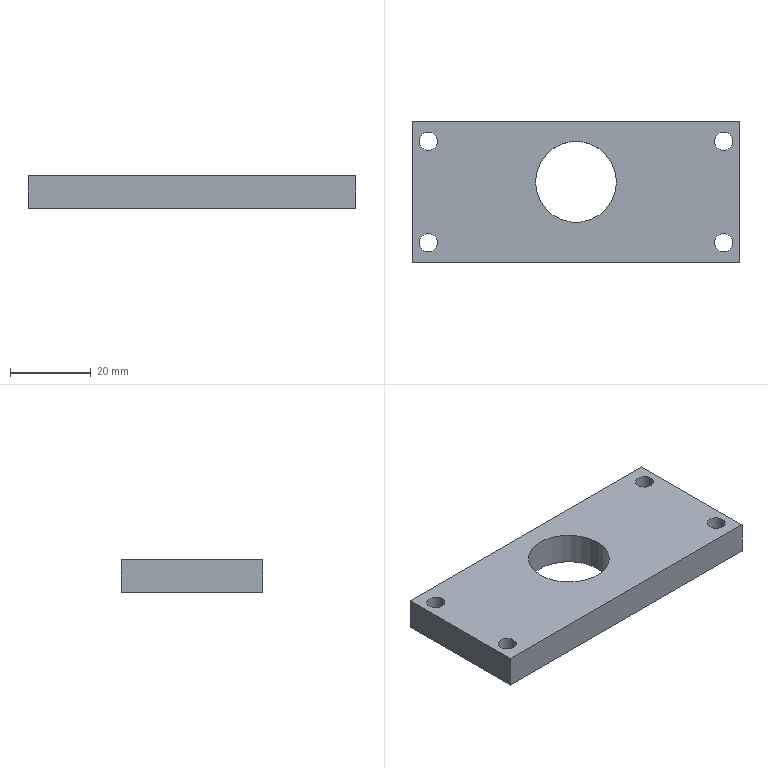Part | STEP file | slingshot push rod cylinder seat | 1 solid | 16 faces | box 81 x 35 x 8 mm | volume 19658 mm3 | cylinder 10 | plane 6 | commonest cylinder face diameters 4.5 x8 20 x2
STEP:
#1=CARTESIAN_POINT('',(0.,0.,0.));
#2=DIRECTION('',(0.,0.,1.));
#3=DIRECTION('',(1.,0.,0.));
#4=AXIS2_PLACEMENT_3D('',#1,#2,#3);
#5=CARTESIAN_POINT('',(-34.25,10.,0.));
#6=VERTEX_POINT('',#5);
#7=CARTESIAN_POINT('',(-34.25,10.,8.));
#8=VERTEX_POINT('',#7);
#9=CARTESIAN_POINT('',(-34.25,10.,-2.));
#10=DIRECTION('',(0.,0.,1.));
#11=VECTOR('',#10,1.);
#12=LINE('',#9,#11);
#13=CARTESIAN_POINT('',(-36.5,10.,-2.));
#14=DIRECTION('',(0.,0.,1.));
#15=DIRECTION('',(1.,0.,0.));
#16=AXIS2_PLACEMENT_3D('',#13,#14,#15);
#17=CYLINDRICAL_SURFACE('',#16,2.25);
#18=CARTESIAN_POINT('',(6.283,0.));
#19=DIRECTION('',(0.,1.));
#20=VECTOR('',#19,1.);
#21=LINE('',#18,#20);
#22=(GEOMETRIC_REPRESENTATION_CONTEXT(2)PARAMETRIC_REPRESENTATION_CONTEXT()REPRESENTATION_CONTEXT('',''));
#23=DEFINITIONAL_REPRESENTATION('',(#21),#22);
#24=PCURVE('',#17,#23);
#25=CARTESIAN_POINT('',(-36.5,10.,-2.));
#26=DIRECTION('',(0.,0.,1.));
#27=DIRECTION('',(1.,0.,0.));
#28=AXIS2_PLACEMENT_3D('',#25,#26,#27);
#29=CYLINDRICAL_SURFACE('',#28,2.25);
#30=CARTESIAN_POINT('',(0.,0.));
#31=DIRECTION('',(0.,1.));
#32=VECTOR('',#31,1.);
#33=LINE('',#30,#32);
#34=(GEOMETRIC_REPRESENTATION_CONTEXT(2)PARAMETRIC_REPRESENTATION_CONTEXT()REPRESENTATION_CONTEXT('',''));
#35=DEFINITIONAL_REPRESENTATION('',(#33),#34);
#36=PCURVE('',#29,#35);
#37=SURFACE_CURVE('',#12,(#24,#36),.PCURVE_S1.);
#38=EDGE_CURVE('',#6,#8,#37,.T.);
#39=ORIENTED_EDGE('',*,*,#38,.T.);
#40=CARTESIAN_POINT('',(-38.75,10.,8.));
#41=VERTEX_POINT('',#40);
#42=CARTESIAN_POINT('',(-36.5,10.,8.));
#43=DIRECTION('',(0.,0.,1.));
#44=DIRECTION('',(1.,0.,0.));
#45=AXIS2_PLACEMENT_3D('',#42,#43,#44);
#46=CIRCLE('',#45,2.25);
#47=CARTESIAN_POINT('',(0.,10.));
#48=DIRECTION('',(1.,0.));
#49=VECTOR('',#48,1.);
#50=LINE('',#47,#49);
#51=(GEOMETRIC_REPRESENTATION_CONTEXT(2)PARAMETRIC_REPRESENTATION_CONTEXT()REPRESENTATION_CONTEXT('',''));
#52=DEFINITIONAL_REPRESENTATION('',(#50),#51);
#53=PCURVE('',#17,#52);
#54=CARTESIAN_POINT('',(-40.5,-20.,8.));
#55=DIRECTION('',(0.,0.,1.));
#56=DIRECTION('',(1.,0.,0.));
#57=AXIS2_PLACEMENT_3D('',#54,#55,#56);
#58=PLANE('',#57);
#59=CARTESIAN_POINT('',(4.,30.));
#60=DIRECTION('',(1.,0.));
#61=AXIS2_PLACEMENT_2D('',#59,#60);
#62=CIRCLE('',#61,2.25);
#63=(GEOMETRIC_REPRESENTATION_CONTEXT(2)PARAMETRIC_REPRESENTATION_CONTEXT()REPRESENTATION_CONTEXT('',''));
#64=DEFINITIONAL_REPRESENTATION('',(#62),#63);
#65=PCURVE('',#58,#64);
#66=SURFACE_CURVE('',#46,(#53,#65),.PCURVE_S1.);
#67=EDGE_CURVE('',#41,#8,#66,.T.);
#68=ORIENTED_EDGE('',*,*,#67,.F.);
#69=CARTESIAN_POINT('',(-38.75,10.,0.));
#70=VERTEX_POINT('',#69);
#71=CARTESIAN_POINT('',(-38.75,10.,-2.));
#72=DIRECTION('',(0.,0.,1.));
#73=VECTOR('',#72,1.);
#74=LINE('',#71,#73);
#75=CARTESIAN_POINT('',(3.142,0.));
#76=DIRECTION('',(0.,1.));
#77=VECTOR('',#76,1.);
#78=LINE('',#75,#77);
#79=(GEOMETRIC_REPRESENTATION_CONTEXT(2)PARAMETRIC_REPRESENTATION_CONTEXT()REPRESENTATION_CONTEXT('',''));
#80=DEFINITIONAL_REPRESENTATION('',(#78),#79);
#81=PCURVE('',#17,#80);
#82=CARTESIAN_POINT('',(3.142,0.));
#83=DIRECTION('',(0.,1.));
#84=VECTOR('',#83,1.);
#85=LINE('',#82,#84);
#86=(GEOMETRIC_REPRESENTATION_CONTEXT(2)PARAMETRIC_REPRESENTATION_CONTEXT()REPRESENTATION_CONTEXT('',''));
#87=DEFINITIONAL_REPRESENTATION('',(#85),#86);
#88=PCURVE('',#29,#87);
#89=SURFACE_CURVE('',#74,(#81,#88),.PCURVE_S1.);
#90=EDGE_CURVE('',#70,#41,#89,.T.);
#91=ORIENTED_EDGE('',*,*,#90,.F.);
#92=CARTESIAN_POINT('',(-36.5,10.,0.));
#93=DIRECTION('',(0.,0.,1.));
#94=DIRECTION('',(1.,0.,0.));
#95=AXIS2_PLACEMENT_3D('',#92,#93,#94);
#96=CIRCLE('',#95,2.25);
#97=CARTESIAN_POINT('',(0.,2.));
#98=DIRECTION('',(1.,0.));
#99=VECTOR('',#98,1.);
#100=LINE('',#97,#99);
#101=(GEOMETRIC_REPRESENTATION_CONTEXT(2)PARAMETRIC_REPRESENTATION_CONTEXT()REPRESENTATION_CONTEXT('',''));
#102=DEFINITIONAL_REPRESENTATION('',(#100),#101);
#103=PCURVE('',#17,#102);
#104=CARTESIAN_POINT('',(-40.5,-20.,0.));
#105=DIRECTION('',(0.,0.,1.));
#106=DIRECTION('',(1.,0.,0.));
#107=AXIS2_PLACEMENT_3D('',#104,#105,#106);
#108=PLANE('',#107);
#109=CARTESIAN_POINT('',(4.,30.));
#110=DIRECTION('',(1.,0.));
#111=AXIS2_PLACEMENT_2D('',#109,#110);
#112=CIRCLE('',#111,2.25);
#113=(GEOMETRIC_REPRESENTATION_CONTEXT(2)PARAMETRIC_REPRESENTATION_CONTEXT()REPRESENTATION_CONTEXT('',''));
#114=DEFINITIONAL_REPRESENTATION('',(#112),#113);
#115=PCURVE('',#108,#114);
#116=SURFACE_CURVE('',#96,(#103,#115),.PCURVE_S1.);
#117=EDGE_CURVE('',#70,#6,#116,.T.);
#118=ORIENTED_EDGE('',*,*,#117,.T.);
#119=EDGE_LOOP('',(#39,#68,#91,#118));
#120=FACE_BOUND('',#119,.F.);
#121=ADVANCED_FACE('',(#120),#17,.F.);
#122=CARTESIAN_POINT('',(-34.25,-15.,0.));
#123=VERTEX_POINT('',#122);
#124=CARTESIAN_POINT('',(-34.25,-15.,8.));
#125=VERTEX_POINT('',#124);
#126=CARTESIAN_POINT('',(-34.25,-15.,-2.));
#127=DIRECTION('',(0.,0.,1.));
#128=VECTOR('',#127,1.);
#129=LINE('',#126,#128);
#130=CARTESIAN_POINT('',(-36.5,-15.,-2.));
#131=DIRECTION('',(0.,0.,1.));
#132=DIRECTION('',(1.,0.,0.));
#133=AXIS2_PLACEMENT_3D('',#130,#131,#132);
#134=CYLINDRICAL_SURFACE('',#133,2.25);
#135=CARTESIAN_POINT('',(6.283,0.));
#136=DIRECTION('',(0.,1.));
#137=VECTOR('',#136,1.);
#138=LINE('',#135,#137);
#139=(GEOMETRIC_REPRESENTATION_CONTEXT(2)PARAMETRIC_REPRESENTATION_CONTEXT()REPRESENTATION_CONTEXT('',''));
#140=DEFINITIONAL_REPRESENTATION('',(#138),#139);
#141=PCURVE('',#134,#140);
#142=CARTESIAN_POINT('',(-36.5,-15.,-2.));
#143=DIRECTION('',(0.,0.,1.));
#144=DIRECTION('',(1.,0.,0.));
#145=AXIS2_PLACEMENT_3D('',#142,#143,#144);
#146=CYLINDRICAL_SURFACE('',#145,2.25);
#147=CARTESIAN_POINT('',(0.,0.));
#148=DIRECTION('',(0.,1.));
#149=VECTOR('',#148,1.);
#150=LINE('',#147,#149);
#151=(GEOMETRIC_REPRESENTATION_CONTEXT(2)PARAMETRIC_REPRESENTATION_CONTEXT()REPRESENTATION_CONTEXT('',''));
#152=DEFINITIONAL_REPRESENTATION('',(#150),#151);
#153=PCURVE('',#146,#152);
#154=SURFACE_CURVE('',#129,(#141,#153),.PCURVE_S1.);
#155=EDGE_CURVE('',#123,#125,#154,.T.);
#156=ORIENTED_EDGE('',*,*,#155,.T.);
#157=CARTESIAN_POINT('',(-38.75,-15.,8.));
#158=VERTEX_POINT('',#157);
#159=CARTESIAN_POINT('',(-36.5,-15.,8.));
#160=DIRECTION('',(0.,0.,1.));
#161=DIRECTION('',(1.,0.,0.));
#162=AXIS2_PLACEMENT_3D('',#159,#160,#161);
#163=CIRCLE('',#162,2.25);
#164=CARTESIAN_POINT('',(0.,10.));
#165=DIRECTION('',(1.,0.));
#166=VECTOR('',#165,1.);
#167=LINE('',#164,#166);
#168=(GEOMETRIC_REPRESENTATION_CONTEXT(2)PARAMETRIC_REPRESENTATION_CONTEXT()REPRESENTATION_CONTEXT('',''));
#169=DEFINITIONAL_REPRESENTATION('',(#167),#168);
#170=PCURVE('',#134,#169);
#171=CARTESIAN_POINT('',(4.,5.));
#172=DIRECTION('',(1.,0.));
#173=AXIS2_PLACEMENT_2D('',#171,#172);
#174=CIRCLE('',#173,2.25);
#175=(GEOMETRIC_REPRESENTATION_CONTEXT(2)PARAMETRIC_REPRESENTATION_CONTEXT()REPRESENTATION_CONTEXT('',''));
#176=DEFINITIONAL_REPRESENTATION('',(#174),#175);
#177=PCURVE('',#58,#176);
#178=SURFACE_CURVE('',#163,(#170,#177),.PCURVE_S1.);
#179=EDGE_CURVE('',#158,#125,#178,.T.);
#180=ORIENTED_EDGE('',*,*,#179,.F.);
#181=CARTESIAN_POINT('',(-38.75,-15.,0.));
#182=VERTEX_POINT('',#181);
#183=CARTESIAN_POINT('',(-38.75,-15.,-2.));
#184=DIRECTION('',(0.,0.,1.));
#185=VECTOR('',#184,1.);
#186=LINE('',#183,#185);
#187=CARTESIAN_POINT('',(3.142,0.));
#188=DIRECTION('',(0.,1.));
#189=VECTOR('',#188,1.);
#190=LINE('',#187,#189);
#191=(GEOMETRIC_REPRESENTATION_CONTEXT(2)PARAMETRIC_REPRESENTATION_CONTEXT()REPRESENTATION_CONTEXT('',''));
#192=DEFINITIONAL_REPRESENTATION('',(#190),#191);
#193=PCURVE('',#134,#192);
#194=CARTESIAN_POINT('',(3.142,0.));
#195=DIRECTION('',(0.,1.));
#196=VECTOR('',#195,1.);
#197=LINE('',#194,#196);
#198=(GEOMETRIC_REPRESENTATION_CONTEXT(2)PARAMETRIC_REPRESENTATION_CONTEXT()REPRESENTATION_CONTEXT('',''));
#199=DEFINITIONAL_REPRESENTATION('',(#197),#198);
#200=PCURVE('',#146,#199);
#201=SURFACE_CURVE('',#186,(#193,#200),.PCURVE_S1.);
#202=EDGE_CURVE('',#182,#158,#201,.T.);
#203=ORIENTED_EDGE('',*,*,#202,.F.);
#204=CARTESIAN_POINT('',(-36.5,-15.,0.));
#205=DIRECTION('',(0.,0.,1.));
#206=DIRECTION('',(1.,0.,0.));
#207=AXIS2_PLACEMENT_3D('',#204,#205,#206);
#208=CIRCLE('',#207,2.25);
#209=CARTESIAN_POINT('',(0.,2.));
#210=DIRECTION('',(1.,0.));
#211=VECTOR('',#210,1.);
#212=LINE('',#209,#211);
#213=(GEOMETRIC_REPRESENTATION_CONTEXT(2)PARAMETRIC_REPRESENTATION_CONTEXT()REPRESENTATION_CONTEXT('',''));
#214=DEFINITIONAL_REPRESENTATION('',(#212),#213);
#215=PCURVE('',#134,#214);
#216=CARTESIAN_POINT('',(4.,5.));
#217=DIRECTION('',(1.,0.));
#218=AXIS2_PLACEMENT_2D('',#216,#217);
#219=CIRCLE('',#218,2.25);
#220=(GEOMETRIC_REPRESENTATION_CONTEXT(2)PARAMETRIC_REPRESENTATION_CONTEXT()REPRESENTATION_CONTEXT('',''));
#221=DEFINITIONAL_REPRESENTATION('',(#219),#220);
#222=PCURVE('',#108,#221);
#223=SURFACE_CURVE('',#208,(#215,#222),.PCURVE_S1.);
#224=EDGE_CURVE('',#182,#123,#223,.T.);
#225=ORIENTED_EDGE('',*,*,#224,.T.);
#226=EDGE_LOOP('',(#156,#180,#203,#225));
#227=FACE_BOUND('',#226,.F.);
#228=ADVANCED_FACE('',(#227),#134,.F.);
#229=CARTESIAN_POINT('',(38.75,-15.,0.));
#230=VERTEX_POINT('',#229);
#231=CARTESIAN_POINT('',(38.75,-15.,8.));
#232=VERTEX_POINT('',#231);
#233=CARTESIAN_POINT('',(38.75,-15.,-2.));
#234=DIRECTION('',(0.,0.,1.));
#235=VECTOR('',#234,1.);
#236=LINE('',#233,#235);
#237=CARTESIAN_POINT('',(36.5,-15.,-2.));
#238=DIRECTION('',(0.,0.,1.));
#239=DIRECTION('',(1.,0.,0.));
#240=AXIS2_PLACEMENT_3D('',#237,#238,#239);
#241=CYLINDRICAL_SURFACE('',#240,2.25);
#242=CARTESIAN_POINT('',(6.283,0.));
#243=DIRECTION('',(0.,1.));
#244=VECTOR('',#243,1.);
#245=LINE('',#242,#244);
#246=(GEOMETRIC_REPRESENTATION_CONTEXT(2)PARAMETRIC_REPRESENTATION_CONTEXT()REPRESENTATION_CONTEXT('',''));
#247=DEFINITIONAL_REPRESENTATION('',(#245),#246);
#248=PCURVE('',#241,#247);
#249=CARTESIAN_POINT('',(36.5,-15.,-2.));
#250=DIRECTION('',(0.,0.,1.));
#251=DIRECTION('',(1.,0.,0.));
#252=AXIS2_PLACEMENT_3D('',#249,#250,#251);
#253=CYLINDRICAL_SURFACE('',#252,2.25);
#254=CARTESIAN_POINT('',(0.,0.));
#255=DIRECTION('',(0.,1.));
#256=VECTOR('',#255,1.);
#257=LINE('',#254,#256);
#258=(GEOMETRIC_REPRESENTATION_CONTEXT(2)PARAMETRIC_REPRESENTATION_CONTEXT()REPRESENTATION_CONTEXT('',''));
#259=DEFINITIONAL_REPRESENTATION('',(#257),#258);
#260=PCURVE('',#253,#259);
#261=SURFACE_CURVE('',#236,(#248,#260),.PCURVE_S1.);
#262=EDGE_CURVE('',#230,#232,#261,.T.);
#263=ORIENTED_EDGE('',*,*,#262,.T.);
#264=CARTESIAN_POINT('',(34.25,-15.,8.));
#265=VERTEX_POINT('',#264);
#266=CARTESIAN_POINT('',(36.5,-15.,8.));
#267=DIRECTION('',(0.,0.,1.));
#268=DIRECTION('',(1.,0.,0.));
#269=AXIS2_PLACEMENT_3D('',#266,#267,#268);
#270=CIRCLE('',#269,2.25);
#271=CARTESIAN_POINT('',(0.,10.));
#272=DIRECTION('',(1.,0.));
#273=VECTOR('',#272,1.);
#274=LINE('',#271,#273);
#275=(GEOMETRIC_REPRESENTATION_CONTEXT(2)PARAMETRIC_REPRESENTATION_CONTEXT()REPRESENTATION_CONTEXT('',''));
#276=DEFINITIONAL_REPRESENTATION('',(#274),#275);
#277=PCURVE('',#241,#276);
#278=CARTESIAN_POINT('',(77.,5.));
#279=DIRECTION('',(1.,0.));
#280=AXIS2_PLACEMENT_2D('',#278,#279);
#281=CIRCLE('',#280,2.25);
#282=(GEOMETRIC_REPRESENTATION_CONTEXT(2)PARAMETRIC_REPRESENTATION_CONTEXT()REPRESENTATION_CONTEXT('',''));
#283=DEFINITIONAL_REPRESENTATION('',(#281),#282);
#284=PCURVE('',#58,#283);
#285=SURFACE_CURVE('',#270,(#277,#284),.PCURVE_S1.);
#286=EDGE_CURVE('',#265,#232,#285,.T.);
#287=ORIENTED_EDGE('',*,*,#286,.F.);
#288=CARTESIAN_POINT('',(34.25,-15.,0.));
#289=VERTEX_POINT('',#288);
#290=CARTESIAN_POINT('',(34.25,-15.,-2.));
#291=DIRECTION('',(0.,0.,1.));
#292=VECTOR('',#291,1.);
#293=LINE('',#290,#292);
#294=CARTESIAN_POINT('',(3.142,0.));
#295=DIRECTION('',(0.,1.));
#296=VECTOR('',#295,1.);
#297=LINE('',#294,#296);
#298=(GEOMETRIC_REPRESENTATION_CONTEXT(2)PARAMETRIC_REPRESENTATION_CONTEXT()REPRESENTATION_CONTEXT('',''));
#299=DEFINITIONAL_REPRESENTATION('',(#297),#298);
#300=PCURVE('',#241,#299);
#301=CARTESIAN_POINT('',(3.142,0.));
#302=DIRECTION('',(0.,1.));
#303=VECTOR('',#302,1.);
#304=LINE('',#301,#303);
#305=(GEOMETRIC_REPRESENTATION_CONTEXT(2)PARAMETRIC_REPRESENTATION_CONTEXT()REPRESENTATION_CONTEXT('',''));
#306=DEFINITIONAL_REPRESENTATION('',(#304),#305);
#307=PCURVE('',#253,#306);
#308=SURFACE_CURVE('',#293,(#300,#307),.PCURVE_S1.);
#309=EDGE_CURVE('',#289,#265,#308,.T.);
#310=ORIENTED_EDGE('',*,*,#309,.F.);
#311=CARTESIAN_POINT('',(36.5,-15.,0.));
#312=DIRECTION('',(0.,0.,1.));
#313=DIRECTION('',(1.,0.,0.));
#314=AXIS2_PLACEMENT_3D('',#311,#312,#313);
#315=CIRCLE('',#314,2.25);
#316=CARTESIAN_POINT('',(0.,2.));
#317=DIRECTION('',(1.,0.));
#318=VECTOR('',#317,1.);
#319=LINE('',#316,#318);
#320=(GEOMETRIC_REPRESENTATION_CONTEXT(2)PARAMETRIC_REPRESENTATION_CONTEXT()REPRESENTATION_CONTEXT('',''));
#321=DEFINITIONAL_REPRESENTATION('',(#319),#320);
#322=PCURVE('',#241,#321);
#323=CARTESIAN_POINT('',(77.,5.));
#324=DIRECTION('',(1.,0.));
#325=AXIS2_PLACEMENT_2D('',#323,#324);
#326=CIRCLE('',#325,2.25);
#327=(GEOMETRIC_REPRESENTATION_CONTEXT(2)PARAMETRIC_REPRESENTATION_CONTEXT()REPRESENTATION_CONTEXT('',''));
#328=DEFINITIONAL_REPRESENTATION('',(#326),#327);
#329=PCURVE('',#108,#328);
#330=SURFACE_CURVE('',#315,(#322,#329),.PCURVE_S1.);
#331=EDGE_CURVE('',#289,#230,#330,.T.);
#332=ORIENTED_EDGE('',*,*,#331,.T.);
#333=EDGE_LOOP('',(#263,#287,#310,#332));
#334=FACE_BOUND('',#333,.F.);
#335=ADVANCED_FACE('',(#334),#241,.F.);
#336=CARTESIAN_POINT('',(38.75,10.,0.));
#337=VERTEX_POINT('',#336);
#338=CARTESIAN_POINT('',(38.75,10.,8.));
#339=VERTEX_POINT('',#338);
#340=CARTESIAN_POINT('',(38.75,10.,-2.));
#341=DIRECTION('',(0.,0.,1.));
#342=VECTOR('',#341,1.);
#343=LINE('',#340,#342);
#344=CARTESIAN_POINT('',(36.5,10.,-2.));
#345=DIRECTION('',(0.,0.,1.));
#346=DIRECTION('',(1.,0.,0.));
#347=AXIS2_PLACEMENT_3D('',#344,#345,#346);
#348=CYLINDRICAL_SURFACE('',#347,2.25);
#349=CARTESIAN_POINT('',(6.283,0.));
#350=DIRECTION('',(0.,1.));
#351=VECTOR('',#350,1.);
#352=LINE('',#349,#351);
#353=(GEOMETRIC_REPRESENTATION_CONTEXT(2)PARAMETRIC_REPRESENTATION_CONTEXT()REPRESENTATION_CONTEXT('',''));
#354=DEFINITIONAL_REPRESENTATION('',(#352),#353);
#355=PCURVE('',#348,#354);
#356=CARTESIAN_POINT('',(36.5,10.,-2.));
#357=DIRECTION('',(0.,0.,1.));
#358=DIRECTION('',(1.,0.,0.));
#359=AXIS2_PLACEMENT_3D('',#356,#357,#358);
#360=CYLINDRICAL_SURFACE('',#359,2.25);
#361=CARTESIAN_POINT('',(0.,0.));
#362=DIRECTION('',(0.,1.));
#363=VECTOR('',#362,1.);
#364=LINE('',#361,#363);
#365=(GEOMETRIC_REPRESENTATION_CONTEXT(2)PARAMETRIC_REPRESENTATION_CONTEXT()REPRESENTATION_CONTEXT('',''));
#366=DEFINITIONAL_REPRESENTATION('',(#364),#365);
#367=PCURVE('',#360,#366);
#368=SURFACE_CURVE('',#343,(#355,#367),.PCURVE_S1.);
#369=EDGE_CURVE('',#337,#339,#368,.T.);
#370=ORIENTED_EDGE('',*,*,#369,.T.);
#371=CARTESIAN_POINT('',(34.25,10.,8.));
#372=VERTEX_POINT('',#371);
#373=CARTESIAN_POINT('',(36.5,10.,8.));
#374=DIRECTION('',(0.,0.,1.));
#375=DIRECTION('',(1.,0.,0.));
#376=AXIS2_PLACEMENT_3D('',#373,#374,#375);
#377=CIRCLE('',#376,2.25);
#378=CARTESIAN_POINT('',(0.,10.));
#379=DIRECTION('',(1.,0.));
#380=VECTOR('',#379,1.);
#381=LINE('',#378,#380);
#382=(GEOMETRIC_REPRESENTATION_CONTEXT(2)PARAMETRIC_REPRESENTATION_CONTEXT()REPRESENTATION_CONTEXT('',''));
#383=DEFINITIONAL_REPRESENTATION('',(#381),#382);
#384=PCURVE('',#348,#383);
#385=CARTESIAN_POINT('',(77.,30.));
#386=DIRECTION('',(1.,0.));
#387=AXIS2_PLACEMENT_2D('',#385,#386);
#388=CIRCLE('',#387,2.25);
#389=(GEOMETRIC_REPRESENTATION_CONTEXT(2)PARAMETRIC_REPRESENTATION_CONTEXT()REPRESENTATION_CONTEXT('',''));
#390=DEFINITIONAL_REPRESENTATION('',(#388),#389);
#391=PCURVE('',#58,#390);
#392=SURFACE_CURVE('',#377,(#384,#391),.PCURVE_S1.);
#393=EDGE_CURVE('',#372,#339,#392,.T.);
#394=ORIENTED_EDGE('',*,*,#393,.F.);
#395=CARTESIAN_POINT('',(34.25,10.,0.));
#396=VERTEX_POINT('',#395);
#397=CARTESIAN_POINT('',(34.25,10.,-2.));
#398=DIRECTION('',(0.,0.,1.));
#399=VECTOR('',#398,1.);
#400=LINE('',#397,#399);
#401=CARTESIAN_POINT('',(3.142,0.));
#402=DIRECTION('',(0.,1.));
#403=VECTOR('',#402,1.);
#404=LINE('',#401,#403);
#405=(GEOMETRIC_REPRESENTATION_CONTEXT(2)PARAMETRIC_REPRESENTATION_CONTEXT()REPRESENTATION_CONTEXT('',''));
#406=DEFINITIONAL_REPRESENTATION('',(#404),#405);
#407=PCURVE('',#348,#406);
#408=CARTESIAN_POINT('',(3.142,0.));
#409=DIRECTION('',(0.,1.));
#410=VECTOR('',#409,1.);
#411=LINE('',#408,#410);
#412=(GEOMETRIC_REPRESENTATION_CONTEXT(2)PARAMETRIC_REPRESENTATION_CONTEXT()REPRESENTATION_CONTEXT('',''));
#413=DEFINITIONAL_REPRESENTATION('',(#411),#412);
#414=PCURVE('',#360,#413);
#415=SURFACE_CURVE('',#400,(#407,#414),.PCURVE_S1.);
#416=EDGE_CURVE('',#396,#372,#415,.T.);
#417=ORIENTED_EDGE('',*,*,#416,.F.);
#418=CARTESIAN_POINT('',(36.5,10.,0.));
#419=DIRECTION('',(0.,0.,1.));
#420=DIRECTION('',(1.,0.,0.));
#421=AXIS2_PLACEMENT_3D('',#418,#419,#420);
#422=CIRCLE('',#421,2.25);
#423=CARTESIAN_POINT('',(0.,2.));
#424=DIRECTION('',(1.,0.));
#425=VECTOR('',#424,1.);
#426=LINE('',#423,#425);
#427=(GEOMETRIC_REPRESENTATION_CONTEXT(2)PARAMETRIC_REPRESENTATION_CONTEXT()REPRESENTATION_CONTEXT('',''));
#428=DEFINITIONAL_REPRESENTATION('',(#426),#427);
#429=PCURVE('',#348,#428);
#430=CARTESIAN_POINT('',(77.,30.));
#431=DIRECTION('',(1.,0.));
#432=AXIS2_PLACEMENT_2D('',#430,#431);
#433=CIRCLE('',#432,2.25);
#434=(GEOMETRIC_REPRESENTATION_CONTEXT(2)PARAMETRIC_REPRESENTATION_CONTEXT()REPRESENTATION_CONTEXT('',''));
#435=DEFINITIONAL_REPRESENTATION('',(#433),#434);
#436=PCURVE('',#108,#435);
#437=SURFACE_CURVE('',#422,(#429,#436),.PCURVE_S1.);
#438=EDGE_CURVE('',#396,#337,#437,.T.);
#439=ORIENTED_EDGE('',*,*,#438,.T.);
#440=EDGE_LOOP('',(#370,#394,#417,#439));
#441=FACE_BOUND('',#440,.F.);
#442=ADVANCED_FACE('',(#441),#348,.F.);
#443=CARTESIAN_POINT('',(-10.,0.,8.));
#444=VERTEX_POINT('',#443);
#445=CARTESIAN_POINT('',(-10.,0.,0.));
#446=VERTEX_POINT('',#445);
#447=CARTESIAN_POINT('',(-10.,0.,8.));
#448=DIRECTION('',(0.,0.,-1.));
#449=VECTOR('',#448,1.);
#450=LINE('',#447,#449);
#451=CARTESIAN_POINT('',(0.,0.,8.));
#452=DIRECTION('',(0.,0.,-1.));
#453=DIRECTION('',(-1.,0.,0.));
#454=AXIS2_PLACEMENT_3D('',#451,#452,#453);
#455=CYLINDRICAL_SURFACE('',#454,10.);
#456=CARTESIAN_POINT('',(6.283,0.));
#457=DIRECTION('',(0.,1.));
#458=VECTOR('',#457,1.);
#459=LINE('',#456,#458);
#460=(GEOMETRIC_REPRESENTATION_CONTEXT(2)PARAMETRIC_REPRESENTATION_CONTEXT()REPRESENTATION_CONTEXT('',''));
#461=DEFINITIONAL_REPRESENTATION('',(#459),#460);
#462=PCURVE('',#455,#461);
#463=CARTESIAN_POINT('',(0.,0.,8.));
#464=DIRECTION('',(0.,0.,-1.));
#465=DIRECTION('',(-1.,0.,0.));
#466=AXIS2_PLACEMENT_3D('',#463,#464,#465);
#467=CYLINDRICAL_SURFACE('',#466,10.);
#468=CARTESIAN_POINT('',(0.,0.));
#469=DIRECTION('',(0.,1.));
#470=VECTOR('',#469,1.);
#471=LINE('',#468,#470);
#472=(GEOMETRIC_REPRESENTATION_CONTEXT(2)PARAMETRIC_REPRESENTATION_CONTEXT()REPRESENTATION_CONTEXT('',''));
#473=DEFINITIONAL_REPRESENTATION('',(#471),#472);
#474=PCURVE('',#467,#473);
#475=SURFACE_CURVE('',#450,(#462,#474),.PCURVE_S1.);
#476=EDGE_CURVE('',#444,#446,#475,.T.);
#477=ORIENTED_EDGE('',*,*,#476,.T.);
#478=CARTESIAN_POINT('',(10.,0.,0.));
#479=VERTEX_POINT('',#478);
#480=CARTESIAN_POINT('',(0.,0.,0.));
#481=DIRECTION('',(0.,0.,1.));
#482=DIRECTION('',(1.,0.,0.));
#483=AXIS2_PLACEMENT_3D('',#480,#481,#482);
#484=CIRCLE('',#483,10.);
#485=CARTESIAN_POINT('',(9.425,8.));
#486=DIRECTION('',(-1.,0.));
#487=VECTOR('',#486,1.);
#488=LINE('',#485,#487);
#489=(GEOMETRIC_REPRESENTATION_CONTEXT(2)PARAMETRIC_REPRESENTATION_CONTEXT()REPRESENTATION_CONTEXT('',''));
#490=DEFINITIONAL_REPRESENTATION('',(#488),#489);
#491=PCURVE('',#455,#490);
#492=CARTESIAN_POINT('',(40.5,20.));
#493=DIRECTION('',(1.,0.));
#494=AXIS2_PLACEMENT_2D('',#492,#493);
#495=CIRCLE('',#494,10.);
#496=(GEOMETRIC_REPRESENTATION_CONTEXT(2)PARAMETRIC_REPRESENTATION_CONTEXT()REPRESENTATION_CONTEXT('',''));
#497=DEFINITIONAL_REPRESENTATION('',(#495),#496);
#498=PCURVE('',#108,#497);
#499=SURFACE_CURVE('',#484,(#491,#498),.PCURVE_S1.);
#500=EDGE_CURVE('',#446,#479,#499,.T.);
#501=ORIENTED_EDGE('',*,*,#500,.T.);
#502=CARTESIAN_POINT('',(10.,0.,8.));
#503=VERTEX_POINT('',#502);
#504=CARTESIAN_POINT('',(10.,0.,8.));
#505=DIRECTION('',(0.,0.,-1.));
#506=VECTOR('',#505,1.);
#507=LINE('',#504,#506);
#508=CARTESIAN_POINT('',(3.142,0.));
#509=DIRECTION('',(0.,1.));
#510=VECTOR('',#509,1.);
#511=LINE('',#508,#510);
#512=(GEOMETRIC_REPRESENTATION_CONTEXT(2)PARAMETRIC_REPRESENTATION_CONTEXT()REPRESENTATION_CONTEXT('',''));
#513=DEFINITIONAL_REPRESENTATION('',(#511),#512);
#514=PCURVE('',#455,#513);
#515=CARTESIAN_POINT('',(3.142,0.));
#516=DIRECTION('',(0.,1.));
#517=VECTOR('',#516,1.);
#518=LINE('',#515,#517);
#519=(GEOMETRIC_REPRESENTATION_CONTEXT(2)PARAMETRIC_REPRESENTATION_CONTEXT()REPRESENTATION_CONTEXT('',''));
#520=DEFINITIONAL_REPRESENTATION('',(#518),#519);
#521=PCURVE('',#467,#520);
#522=SURFACE_CURVE('',#507,(#514,#521),.PCURVE_S1.);
#523=EDGE_CURVE('',#503,#479,#522,.T.);
#524=ORIENTED_EDGE('',*,*,#523,.F.);
#525=CARTESIAN_POINT('',(0.,0.,8.));
#526=DIRECTION('',(0.,0.,1.));
#527=DIRECTION('',(1.,0.,0.));
#528=AXIS2_PLACEMENT_3D('',#525,#526,#527);
#529=CIRCLE('',#528,10.);
#530=CARTESIAN_POINT('',(9.425,0.));
#531=DIRECTION('',(-1.,0.));
#532=VECTOR('',#531,1.);
#533=LINE('',#530,#532);
#534=(GEOMETRIC_REPRESENTATION_CONTEXT(2)PARAMETRIC_REPRESENTATION_CONTEXT()REPRESENTATION_CONTEXT('',''));
#535=DEFINITIONAL_REPRESENTATION('',(#533),#534);
#536=PCURVE('',#455,#535);
#537=CARTESIAN_POINT('',(40.5,20.));
#538=DIRECTION('',(1.,0.));
#539=AXIS2_PLACEMENT_2D('',#537,#538);
#540=CIRCLE('',#539,10.);
#541=(GEOMETRIC_REPRESENTATION_CONTEXT(2)PARAMETRIC_REPRESENTATION_CONTEXT()REPRESENTATION_CONTEXT('',''));
#542=DEFINITIONAL_REPRESENTATION('',(#540),#541);
#543=PCURVE('',#58,#542);
#544=SURFACE_CURVE('',#529,(#536,#543),.PCURVE_S1.);
#545=EDGE_CURVE('',#444,#503,#544,.T.);
#546=ORIENTED_EDGE('',*,*,#545,.F.);
#547=EDGE_LOOP('',(#477,#501,#524,#546));
#548=FACE_BOUND('',#547,.F.);
#549=ADVANCED_FACE('',(#548),#455,.F.);
#550=CARTESIAN_POINT('',(-36.5,10.,8.));
#551=DIRECTION('',(0.,0.,1.));
#552=DIRECTION('',(1.,0.,0.));
#553=AXIS2_PLACEMENT_3D('',#550,#551,#552);
#554=CIRCLE('',#553,2.25);
#555=CARTESIAN_POINT('',(4.,30.));
#556=DIRECTION('',(1.,0.));
#557=AXIS2_PLACEMENT_2D('',#555,#556);
#558=CIRCLE('',#557,2.25);
#559=(GEOMETRIC_REPRESENTATION_CONTEXT(2)PARAMETRIC_REPRESENTATION_CONTEXT()REPRESENTATION_CONTEXT('',''));
#560=DEFINITIONAL_REPRESENTATION('',(#558),#559);
#561=PCURVE('',#58,#560);
#562=CARTESIAN_POINT('',(0.,10.));
#563=DIRECTION('',(1.,0.));
#564=VECTOR('',#563,1.);
#565=LINE('',#562,#564);
#566=(GEOMETRIC_REPRESENTATION_CONTEXT(2)PARAMETRIC_REPRESENTATION_CONTEXT()REPRESENTATION_CONTEXT('',''));
#567=DEFINITIONAL_REPRESENTATION('',(#565),#566);
#568=PCURVE('',#29,#567);
#569=SURFACE_CURVE('',#554,(#561,#568),.PCURVE_S1.);
#570=EDGE_CURVE('',#8,#41,#569,.T.);
#571=ORIENTED_EDGE('',*,*,#570,.F.);
#572=ORIENTED_EDGE('',*,*,#67,.F.);
#573=EDGE_LOOP('',(#571,#572));
#574=FACE_BOUND('',#573,.T.);
#575=CARTESIAN_POINT('',(-36.5,-15.,8.));
#576=DIRECTION('',(0.,0.,1.));
#577=DIRECTION('',(1.,0.,0.));
#578=AXIS2_PLACEMENT_3D('',#575,#576,#577);
#579=CIRCLE('',#578,2.25);
#580=CARTESIAN_POINT('',(4.,5.));
#581=DIRECTION('',(1.,0.));
#582=AXIS2_PLACEMENT_2D('',#580,#581);
#583=CIRCLE('',#582,2.25);
#584=(GEOMETRIC_REPRESENTATION_CONTEXT(2)PARAMETRIC_REPRESENTATION_CONTEXT()REPRESENTATION_CONTEXT('',''));
#585=DEFINITIONAL_REPRESENTATION('',(#583),#584);
#586=PCURVE('',#58,#585);
#587=CARTESIAN_POINT('',(0.,10.));
#588=DIRECTION('',(1.,0.));
#589=VECTOR('',#588,1.);
#590=LINE('',#587,#589);
#591=(GEOMETRIC_REPRESENTATION_CONTEXT(2)PARAMETRIC_REPRESENTATION_CONTEXT()REPRESENTATION_CONTEXT('',''));
#592=DEFINITIONAL_REPRESENTATION('',(#590),#591);
#593=PCURVE('',#146,#592);
#594=SURFACE_CURVE('',#579,(#586,#593),.PCURVE_S1.);
#595=EDGE_CURVE('',#125,#158,#594,.T.);
#596=ORIENTED_EDGE('',*,*,#595,.F.);
#597=ORIENTED_EDGE('',*,*,#179,.F.);
#598=EDGE_LOOP('',(#596,#597));
#599=FACE_BOUND('',#598,.T.);
#600=CARTESIAN_POINT('',(36.5,-15.,8.));
#601=DIRECTION('',(0.,0.,1.));
#602=DIRECTION('',(1.,0.,0.));
#603=AXIS2_PLACEMENT_3D('',#600,#601,#602);
#604=CIRCLE('',#603,2.25);
#605=CARTESIAN_POINT('',(77.,5.));
#606=DIRECTION('',(1.,0.));
#607=AXIS2_PLACEMENT_2D('',#605,#606);
#608=CIRCLE('',#607,2.25);
#609=(GEOMETRIC_REPRESENTATION_CONTEXT(2)PARAMETRIC_REPRESENTATION_CONTEXT()REPRESENTATION_CONTEXT('',''));
#610=DEFINITIONAL_REPRESENTATION('',(#608),#609);
#611=PCURVE('',#58,#610);
#612=CARTESIAN_POINT('',(0.,10.));
#613=DIRECTION('',(1.,0.));
#614=VECTOR('',#613,1.);
#615=LINE('',#612,#614);
#616=(GEOMETRIC_REPRESENTATION_CONTEXT(2)PARAMETRIC_REPRESENTATION_CONTEXT()REPRESENTATION_CONTEXT('',''));
#617=DEFINITIONAL_REPRESENTATION('',(#615),#616);
#618=PCURVE('',#253,#617);
#619=SURFACE_CURVE('',#604,(#611,#618),.PCURVE_S1.);
#620=EDGE_CURVE('',#232,#265,#619,.T.);
#621=ORIENTED_EDGE('',*,*,#620,.F.);
#622=ORIENTED_EDGE('',*,*,#286,.F.);
#623=EDGE_LOOP('',(#621,#622));
#624=FACE_BOUND('',#623,.T.);
#625=CARTESIAN_POINT('',(36.5,10.,8.));
#626=DIRECTION('',(0.,0.,1.));
#627=DIRECTION('',(1.,0.,0.));
#628=AXIS2_PLACEMENT_3D('',#625,#626,#627);
#629=CIRCLE('',#628,2.25);
#630=CARTESIAN_POINT('',(77.,30.));
#631=DIRECTION('',(1.,0.));
#632=AXIS2_PLACEMENT_2D('',#630,#631);
#633=CIRCLE('',#632,2.25);
#634=(GEOMETRIC_REPRESENTATION_CONTEXT(2)PARAMETRIC_REPRESENTATION_CONTEXT()REPRESENTATION_CONTEXT('',''));
#635=DEFINITIONAL_REPRESENTATION('',(#633),#634);
#636=PCURVE('',#58,#635);
#637=CARTESIAN_POINT('',(0.,10.));
#638=DIRECTION('',(1.,0.));
#639=VECTOR('',#638,1.);
#640=LINE('',#637,#639);
#641=(GEOMETRIC_REPRESENTATION_CONTEXT(2)PARAMETRIC_REPRESENTATION_CONTEXT()REPRESENTATION_CONTEXT('',''));
#642=DEFINITIONAL_REPRESENTATION('',(#640),#641);
#643=PCURVE('',#360,#642);
#644=SURFACE_CURVE('',#629,(#636,#643),.PCURVE_S1.);
#645=EDGE_CURVE('',#339,#372,#644,.T.);
#646=ORIENTED_EDGE('',*,*,#645,.F.);
#647=ORIENTED_EDGE('',*,*,#393,.F.);
#648=EDGE_LOOP('',(#646,#647));
#649=FACE_BOUND('',#648,.T.);
#650=CARTESIAN_POINT('',(-40.5,15.,8.));
#651=VERTEX_POINT('',#650);
#652=CARTESIAN_POINT('',(-40.5,-20.,8.));
#653=VERTEX_POINT('',#652);
#654=CARTESIAN_POINT('',(-40.5,15.,8.));
#655=DIRECTION('',(0.,-1.,0.));
#656=VECTOR('',#655,1.);
#657=LINE('',#654,#656);
#658=CARTESIAN_POINT('',(0.,35.));
#659=DIRECTION('',(0.,-1.));
#660=VECTOR('',#659,1.);
#661=LINE('',#658,#660);
#662=(GEOMETRIC_REPRESENTATION_CONTEXT(2)PARAMETRIC_REPRESENTATION_CONTEXT()REPRESENTATION_CONTEXT('',''));
#663=DEFINITIONAL_REPRESENTATION('',(#661),#662);
#664=PCURVE('',#58,#663);
#665=CARTESIAN_POINT('',(-40.5,15.,8.));
#666=DIRECTION('',(1.,0.,0.));
#667=DIRECTION('',(0.,1.,0.));
#668=AXIS2_PLACEMENT_3D('',#665,#666,#667);
#669=PLANE('',#668);
#670=CARTESIAN_POINT('',(0.,0.));
#671=DIRECTION('',(-1.,0.));
#672=VECTOR('',#671,1.);
#673=LINE('',#670,#672);
#674=(GEOMETRIC_REPRESENTATION_CONTEXT(2)PARAMETRIC_REPRESENTATION_CONTEXT()REPRESENTATION_CONTEXT('',''));
#675=DEFINITIONAL_REPRESENTATION('',(#673),#674);
#676=PCURVE('',#669,#675);
#677=SURFACE_CURVE('',#657,(#664,#676),.PCURVE_S1.);
#678=EDGE_CURVE('',#651,#653,#677,.T.);
#679=ORIENTED_EDGE('',*,*,#678,.T.);
#680=CARTESIAN_POINT('',(40.5,-20.,8.));
#681=VERTEX_POINT('',#680);
#682=CARTESIAN_POINT('',(-40.5,-20.,8.));
#683=DIRECTION('',(1.,0.,0.));
#684=VECTOR('',#683,1.);
#685=LINE('',#682,#684);
#686=CARTESIAN_POINT('',(0.,0.));
#687=DIRECTION('',(1.,0.));
#688=VECTOR('',#687,1.);
#689=LINE('',#686,#688);
#690=(GEOMETRIC_REPRESENTATION_CONTEXT(2)PARAMETRIC_REPRESENTATION_CONTEXT()REPRESENTATION_CONTEXT('',''));
#691=DEFINITIONAL_REPRESENTATION('',(#689),#690);
#692=PCURVE('',#58,#691);
#693=CARTESIAN_POINT('',(-40.5,-20.,8.));
#694=DIRECTION('',(0.,1.,0.));
#695=DIRECTION('',(0.,0.,1.));
#696=AXIS2_PLACEMENT_3D('',#693,#694,#695);
#697=PLANE('',#696);
#698=CARTESIAN_POINT('',(0.,0.));
#699=DIRECTION('',(0.,1.));
#700=VECTOR('',#699,1.);
#701=LINE('',#698,#700);
#702=(GEOMETRIC_REPRESENTATION_CONTEXT(2)PARAMETRIC_REPRESENTATION_CONTEXT()REPRESENTATION_CONTEXT('',''));
#703=DEFINITIONAL_REPRESENTATION('',(#701),#702);
#704=PCURVE('',#697,#703);
#705=SURFACE_CURVE('',#685,(#692,#704),.PCURVE_S1.);
#706=EDGE_CURVE('',#653,#681,#705,.T.);
#707=ORIENTED_EDGE('',*,*,#706,.T.);
#708=CARTESIAN_POINT('',(40.5,15.,8.));
#709=VERTEX_POINT('',#708);
#710=CARTESIAN_POINT('',(40.5,15.,8.));
#711=DIRECTION('',(0.,1.,0.));
#712=VECTOR('',#711,1.);
#713=LINE('',#710,#712);
#714=CARTESIAN_POINT('',(81.,35.));
#715=DIRECTION('',(0.,1.));
#716=VECTOR('',#715,1.);
#717=LINE('',#714,#716);
#718=(GEOMETRIC_REPRESENTATION_CONTEXT(2)PARAMETRIC_REPRESENTATION_CONTEXT()REPRESENTATION_CONTEXT('',''));
#719=DEFINITIONAL_REPRESENTATION('',(#717),#718);
#720=PCURVE('',#58,#719);
#721=CARTESIAN_POINT('',(40.5,15.,8.));
#722=DIRECTION('',(-1.,0.,0.));
#723=DIRECTION('',(0.,-1.,0.));
#724=AXIS2_PLACEMENT_3D('',#721,#722,#723);
#725=PLANE('',#724);
#726=CARTESIAN_POINT('',(0.,0.));
#727=DIRECTION('',(-1.,0.));
#728=VECTOR('',#727,1.);
#729=LINE('',#726,#728);
#730=(GEOMETRIC_REPRESENTATION_CONTEXT(2)PARAMETRIC_REPRESENTATION_CONTEXT()REPRESENTATION_CONTEXT('',''));
#731=DEFINITIONAL_REPRESENTATION('',(#729),#730);
#732=PCURVE('',#725,#731);
#733=SURFACE_CURVE('',#713,(#720,#732),.PCURVE_S1.);
#734=EDGE_CURVE('',#681,#709,#733,.T.);
#735=ORIENTED_EDGE('',*,*,#734,.T.);
#736=CARTESIAN_POINT('',(-40.5,15.,8.));
#737=DIRECTION('',(-1.,0.,0.));
#738=VECTOR('',#737,1.);
#739=LINE('',#736,#738);
#740=CARTESIAN_POINT('',(0.,35.));
#741=DIRECTION('',(-1.,0.));
#742=VECTOR('',#741,1.);
#743=LINE('',#740,#742);
#744=(GEOMETRIC_REPRESENTATION_CONTEXT(2)PARAMETRIC_REPRESENTATION_CONTEXT()REPRESENTATION_CONTEXT('',''));
#745=DEFINITIONAL_REPRESENTATION('',(#743),#744);
#746=PCURVE('',#58,#745);
#747=CARTESIAN_POINT('',(-40.5,15.,8.));
#748=DIRECTION('',(0.,-1.,0.));
#749=DIRECTION('',(0.,0.,-1.));
#750=AXIS2_PLACEMENT_3D('',#747,#748,#749);
#751=PLANE('',#750);
#752=CARTESIAN_POINT('',(0.,0.));
#753=DIRECTION('',(0.,-1.));
#754=VECTOR('',#753,1.);
#755=LINE('',#752,#754);
#756=(GEOMETRIC_REPRESENTATION_CONTEXT(2)PARAMETRIC_REPRESENTATION_CONTEXT()REPRESENTATION_CONTEXT('',''));
#757=DEFINITIONAL_REPRESENTATION('',(#755),#756);
#758=PCURVE('',#751,#757);
#759=SURFACE_CURVE('',#739,(#746,#758),.PCURVE_S1.);
#760=EDGE_CURVE('',#709,#651,#759,.T.);
#761=ORIENTED_EDGE('',*,*,#760,.T.);
#762=EDGE_LOOP('',(#679,#707,#735,#761));
#763=FACE_BOUND('',#762,.T.);
#764=ORIENTED_EDGE('',*,*,#545,.F.);
#765=CARTESIAN_POINT('',(0.,0.,8.));
#766=DIRECTION('',(0.,0.,1.));
#767=DIRECTION('',(1.,0.,0.));
#768=AXIS2_PLACEMENT_3D('',#765,#766,#767);
#769=CIRCLE('',#768,10.);
#770=CARTESIAN_POINT('',(40.5,20.));
#771=DIRECTION('',(1.,0.));
#772=AXIS2_PLACEMENT_2D('',#770,#771);
#773=CIRCLE('',#772,10.);
#774=(GEOMETRIC_REPRESENTATION_CONTEXT(2)PARAMETRIC_REPRESENTATION_CONTEXT()REPRESENTATION_CONTEXT('',''));
#775=DEFINITIONAL_REPRESENTATION('',(#773),#774);
#776=PCURVE('',#58,#775);
#777=CARTESIAN_POINT('',(3.142,0.));
#778=DIRECTION('',(-1.,0.));
#779=VECTOR('',#778,1.);
#780=LINE('',#777,#779);
#781=(GEOMETRIC_REPRESENTATION_CONTEXT(2)PARAMETRIC_REPRESENTATION_CONTEXT()REPRESENTATION_CONTEXT('',''));
#782=DEFINITIONAL_REPRESENTATION('',(#780),#781);
#783=PCURVE('',#467,#782);
#784=SURFACE_CURVE('',#769,(#776,#783),.PCURVE_S1.);
#785=EDGE_CURVE('',#503,#444,#784,.T.);
#786=ORIENTED_EDGE('',*,*,#785,.F.);
#787=EDGE_LOOP('',(#764,#786));
#788=FACE_BOUND('',#787,.T.);
#789=ADVANCED_FACE('',(#574,#599,#624,#649,#763,#788),#58,.T.);
#790=CARTESIAN_POINT('',(-36.5,10.,0.));
#791=DIRECTION('',(0.,0.,1.));
#792=DIRECTION('',(1.,0.,0.));
#793=AXIS2_PLACEMENT_3D('',#790,#791,#792);
#794=CIRCLE('',#793,2.25);
#795=CARTESIAN_POINT('',(4.,30.));
#796=DIRECTION('',(1.,0.));
#797=AXIS2_PLACEMENT_2D('',#795,#796);
#798=CIRCLE('',#797,2.25);
#799=(GEOMETRIC_REPRESENTATION_CONTEXT(2)PARAMETRIC_REPRESENTATION_CONTEXT()REPRESENTATION_CONTEXT('',''));
#800=DEFINITIONAL_REPRESENTATION('',(#798),#799);
#801=PCURVE('',#108,#800);
#802=CARTESIAN_POINT('',(0.,2.));
#803=DIRECTION('',(1.,0.));
#804=VECTOR('',#803,1.);
#805=LINE('',#802,#804);
#806=(GEOMETRIC_REPRESENTATION_CONTEXT(2)PARAMETRIC_REPRESENTATION_CONTEXT()REPRESENTATION_CONTEXT('',''));
#807=DEFINITIONAL_REPRESENTATION('',(#805),#806);
#808=PCURVE('',#29,#807);
#809=SURFACE_CURVE('',#794,(#801,#808),.PCURVE_S1.);
#810=EDGE_CURVE('',#6,#70,#809,.T.);
#811=ORIENTED_EDGE('',*,*,#810,.T.);
#812=ORIENTED_EDGE('',*,*,#117,.T.);
#813=EDGE_LOOP('',(#811,#812));
#814=FACE_BOUND('',#813,.T.);
#815=CARTESIAN_POINT('',(-36.5,-15.,0.));
#816=DIRECTION('',(0.,0.,1.));
#817=DIRECTION('',(1.,0.,0.));
#818=AXIS2_PLACEMENT_3D('',#815,#816,#817);
#819=CIRCLE('',#818,2.25);
#820=CARTESIAN_POINT('',(4.,5.));
#821=DIRECTION('',(1.,0.));
#822=AXIS2_PLACEMENT_2D('',#820,#821);
#823=CIRCLE('',#822,2.25);
#824=(GEOMETRIC_REPRESENTATION_CONTEXT(2)PARAMETRIC_REPRESENTATION_CONTEXT()REPRESENTATION_CONTEXT('',''));
#825=DEFINITIONAL_REPRESENTATION('',(#823),#824);
#826=PCURVE('',#108,#825);
#827=CARTESIAN_POINT('',(0.,2.));
#828=DIRECTION('',(1.,0.));
#829=VECTOR('',#828,1.);
#830=LINE('',#827,#829);
#831=(GEOMETRIC_REPRESENTATION_CONTEXT(2)PARAMETRIC_REPRESENTATION_CONTEXT()REPRESENTATION_CONTEXT('',''));
#832=DEFINITIONAL_REPRESENTATION('',(#830),#831);
#833=PCURVE('',#146,#832);
#834=SURFACE_CURVE('',#819,(#826,#833),.PCURVE_S1.);
#835=EDGE_CURVE('',#123,#182,#834,.T.);
#836=ORIENTED_EDGE('',*,*,#835,.T.);
#837=ORIENTED_EDGE('',*,*,#224,.T.);
#838=EDGE_LOOP('',(#836,#837));
#839=FACE_BOUND('',#838,.T.);
#840=CARTESIAN_POINT('',(36.5,-15.,0.));
#841=DIRECTION('',(0.,0.,1.));
#842=DIRECTION('',(1.,0.,0.));
#843=AXIS2_PLACEMENT_3D('',#840,#841,#842);
#844=CIRCLE('',#843,2.25);
#845=CARTESIAN_POINT('',(77.,5.));
#846=DIRECTION('',(1.,0.));
#847=AXIS2_PLACEMENT_2D('',#845,#846);
#848=CIRCLE('',#847,2.25);
#849=(GEOMETRIC_REPRESENTATION_CONTEXT(2)PARAMETRIC_REPRESENTATION_CONTEXT()REPRESENTATION_CONTEXT('',''));
#850=DEFINITIONAL_REPRESENTATION('',(#848),#849);
#851=PCURVE('',#108,#850);
#852=CARTESIAN_POINT('',(0.,2.));
#853=DIRECTION('',(1.,0.));
#854=VECTOR('',#853,1.);
#855=LINE('',#852,#854);
#856=(GEOMETRIC_REPRESENTATION_CONTEXT(2)PARAMETRIC_REPRESENTATION_CONTEXT()REPRESENTATION_CONTEXT('',''));
#857=DEFINITIONAL_REPRESENTATION('',(#855),#856);
#858=PCURVE('',#253,#857);
#859=SURFACE_CURVE('',#844,(#851,#858),.PCURVE_S1.);
#860=EDGE_CURVE('',#230,#289,#859,.T.);
#861=ORIENTED_EDGE('',*,*,#860,.T.);
#862=ORIENTED_EDGE('',*,*,#331,.T.);
#863=EDGE_LOOP('',(#861,#862));
#864=FACE_BOUND('',#863,.T.);
#865=CARTESIAN_POINT('',(36.5,10.,0.));
#866=DIRECTION('',(0.,0.,1.));
#867=DIRECTION('',(1.,0.,0.));
#868=AXIS2_PLACEMENT_3D('',#865,#866,#867);
#869=CIRCLE('',#868,2.25);
#870=CARTESIAN_POINT('',(77.,30.));
#871=DIRECTION('',(1.,0.));
#872=AXIS2_PLACEMENT_2D('',#870,#871);
#873=CIRCLE('',#872,2.25);
#874=(GEOMETRIC_REPRESENTATION_CONTEXT(2)PARAMETRIC_REPRESENTATION_CONTEXT()REPRESENTATION_CONTEXT('',''));
#875=DEFINITIONAL_REPRESENTATION('',(#873),#874);
#876=PCURVE('',#108,#875);
#877=CARTESIAN_POINT('',(0.,2.));
#878=DIRECTION('',(1.,0.));
#879=VECTOR('',#878,1.);
#880=LINE('',#877,#879);
#881=(GEOMETRIC_REPRESENTATION_CONTEXT(2)PARAMETRIC_REPRESENTATION_CONTEXT()REPRESENTATION_CONTEXT('',''));
#882=DEFINITIONAL_REPRESENTATION('',(#880),#881);
#883=PCURVE('',#360,#882);
#884=SURFACE_CURVE('',#869,(#876,#883),.PCURVE_S1.);
#885=EDGE_CURVE('',#337,#396,#884,.T.);
#886=ORIENTED_EDGE('',*,*,#885,.T.);
#887=ORIENTED_EDGE('',*,*,#438,.T.);
#888=EDGE_LOOP('',(#886,#887));
#889=FACE_BOUND('',#888,.T.);
#890=CARTESIAN_POINT('',(-40.5,15.,0.));
#891=VERTEX_POINT('',#890);
#892=CARTESIAN_POINT('',(-40.5,-20.,0.));
#893=VERTEX_POINT('',#892);
#894=CARTESIAN_POINT('',(-40.5,15.,0.));
#895=DIRECTION('',(0.,-1.,0.));
#896=VECTOR('',#895,1.);
#897=LINE('',#894,#896);
#898=CARTESIAN_POINT('',(0.,35.));
#899=DIRECTION('',(0.,-1.));
#900=VECTOR('',#899,1.);
#901=LINE('',#898,#900);
#902=(GEOMETRIC_REPRESENTATION_CONTEXT(2)PARAMETRIC_REPRESENTATION_CONTEXT()REPRESENTATION_CONTEXT('',''));
#903=DEFINITIONAL_REPRESENTATION('',(#901),#902);
#904=PCURVE('',#108,#903);
#905=CARTESIAN_POINT('',(0.,-8.));
#906=DIRECTION('',(-1.,0.));
#907=VECTOR('',#906,1.);
#908=LINE('',#905,#907);
#909=(GEOMETRIC_REPRESENTATION_CONTEXT(2)PARAMETRIC_REPRESENTATION_CONTEXT()REPRESENTATION_CONTEXT('',''));
#910=DEFINITIONAL_REPRESENTATION('',(#908),#909);
#911=PCURVE('',#669,#910);
#912=SURFACE_CURVE('',#897,(#904,#911),.PCURVE_S1.);
#913=EDGE_CURVE('',#891,#893,#912,.T.);
#914=ORIENTED_EDGE('',*,*,#913,.F.);
#915=CARTESIAN_POINT('',(40.5,15.,0.));
#916=VERTEX_POINT('',#915);
#917=CARTESIAN_POINT('',(-40.5,15.,0.));
#918=DIRECTION('',(-1.,0.,0.));
#919=VECTOR('',#918,1.);
#920=LINE('',#917,#919);
#921=CARTESIAN_POINT('',(0.,35.));
#922=DIRECTION('',(-1.,0.));
#923=VECTOR('',#922,1.);
#924=LINE('',#921,#923);
#925=(GEOMETRIC_REPRESENTATION_CONTEXT(2)PARAMETRIC_REPRESENTATION_CONTEXT()REPRESENTATION_CONTEXT('',''));
#926=DEFINITIONAL_REPRESENTATION('',(#924),#925);
#927=PCURVE('',#108,#926);
#928=CARTESIAN_POINT('',(8.,0.));
#929=DIRECTION('',(0.,-1.));
#930=VECTOR('',#929,1.);
#931=LINE('',#928,#930);
#932=(GEOMETRIC_REPRESENTATION_CONTEXT(2)PARAMETRIC_REPRESENTATION_CONTEXT()REPRESENTATION_CONTEXT('',''));
#933=DEFINITIONAL_REPRESENTATION('',(#931),#932);
#934=PCURVE('',#751,#933);
#935=SURFACE_CURVE('',#920,(#927,#934),.PCURVE_S1.);
#936=EDGE_CURVE('',#916,#891,#935,.T.);
#937=ORIENTED_EDGE('',*,*,#936,.F.);
#938=CARTESIAN_POINT('',(40.5,-20.,0.));
#939=VERTEX_POINT('',#938);
#940=CARTESIAN_POINT('',(40.5,15.,0.));
#941=DIRECTION('',(0.,1.,0.));
#942=VECTOR('',#941,1.);
#943=LINE('',#940,#942);
#944=CARTESIAN_POINT('',(81.,35.));
#945=DIRECTION('',(0.,1.));
#946=VECTOR('',#945,1.);
#947=LINE('',#944,#946);
#948=(GEOMETRIC_REPRESENTATION_CONTEXT(2)PARAMETRIC_REPRESENTATION_CONTEXT()REPRESENTATION_CONTEXT('',''));
#949=DEFINITIONAL_REPRESENTATION('',(#947),#948);
#950=PCURVE('',#108,#949);
#951=CARTESIAN_POINT('',(0.,-8.));
#952=DIRECTION('',(-1.,0.));
#953=VECTOR('',#952,1.);
#954=LINE('',#951,#953);
#955=(GEOMETRIC_REPRESENTATION_CONTEXT(2)PARAMETRIC_REPRESENTATION_CONTEXT()REPRESENTATION_CONTEXT('',''));
#956=DEFINITIONAL_REPRESENTATION('',(#954),#955);
#957=PCURVE('',#725,#956);
#958=SURFACE_CURVE('',#943,(#950,#957),.PCURVE_S1.);
#959=EDGE_CURVE('',#939,#916,#958,.T.);
#960=ORIENTED_EDGE('',*,*,#959,.F.);
#961=CARTESIAN_POINT('',(-40.5,-20.,0.));
#962=DIRECTION('',(1.,0.,0.));
#963=VECTOR('',#962,1.);
#964=LINE('',#961,#963);
#965=CARTESIAN_POINT('',(0.,0.));
#966=DIRECTION('',(1.,0.));
#967=VECTOR('',#966,1.);
#968=LINE('',#965,#967);
#969=(GEOMETRIC_REPRESENTATION_CONTEXT(2)PARAMETRIC_REPRESENTATION_CONTEXT()REPRESENTATION_CONTEXT('',''));
#970=DEFINITIONAL_REPRESENTATION('',(#968),#969);
#971=PCURVE('',#108,#970);
#972=CARTESIAN_POINT('',(-8.,0.));
#973=DIRECTION('',(0.,1.));
#974=VECTOR('',#973,1.);
#975=LINE('',#972,#974);
#976=(GEOMETRIC_REPRESENTATION_CONTEXT(2)PARAMETRIC_REPRESENTATION_CONTEXT()REPRESENTATION_CONTEXT('',''));
#977=DEFINITIONAL_REPRESENTATION('',(#975),#976);
#978=PCURVE('',#697,#977);
#979=SURFACE_CURVE('',#964,(#971,#978),.PCURVE_S1.);
#980=EDGE_CURVE('',#893,#939,#979,.T.);
#981=ORIENTED_EDGE('',*,*,#980,.F.);
#982=EDGE_LOOP('',(#914,#937,#960,#981));
#983=FACE_BOUND('',#982,.T.);
#984=ORIENTED_EDGE('',*,*,#500,.T.);
#985=CARTESIAN_POINT('',(0.,0.,0.));
#986=DIRECTION('',(0.,0.,1.));
#987=DIRECTION('',(1.,0.,0.));
#988=AXIS2_PLACEMENT_3D('',#985,#986,#987);
#989=CIRCLE('',#988,10.);
#990=CARTESIAN_POINT('',(40.5,20.));
#991=DIRECTION('',(1.,0.));
#992=AXIS2_PLACEMENT_2D('',#990,#991);
#993=CIRCLE('',#992,10.);
#994=(GEOMETRIC_REPRESENTATION_CONTEXT(2)PARAMETRIC_REPRESENTATION_CONTEXT()REPRESENTATION_CONTEXT('',''));
#995=DEFINITIONAL_REPRESENTATION('',(#993),#994);
#996=PCURVE('',#108,#995);
#997=CARTESIAN_POINT('',(3.142,8.));
#998=DIRECTION('',(-1.,0.));
#999=VECTOR('',#998,1.);
#1000=LINE('',#997,#999);
#1001=(GEOMETRIC_REPRESENTATION_CONTEXT(2)PARAMETRIC_REPRESENTATION_CONTEXT()REPRESENTATION_CONTEXT('',''));
#1002=DEFINITIONAL_REPRESENTATION('',(#1000),#1001);
#1003=PCURVE('',#467,#1002);
#1004=SURFACE_CURVE('',#989,(#996,#1003),.PCURVE_S1.);
#1005=EDGE_CURVE('',#479,#446,#1004,.T.);
#1006=ORIENTED_EDGE('',*,*,#1005,.T.);
#1007=EDGE_LOOP('',(#984,#1006));
#1008=FACE_BOUND('',#1007,.T.);
#1009=ADVANCED_FACE('',(#814,#839,#864,#889,#983,#1008),#108,.F.);
#1010=ORIENTED_EDGE('',*,*,#913,.T.);
#1011=CARTESIAN_POINT('',(-40.5,-20.,8.));
#1012=DIRECTION('',(0.,0.,-1.));
#1013=VECTOR('',#1012,1.);
#1014=LINE('',#1011,#1013);
#1015=CARTESIAN_POINT('',(-35.,0.));
#1016=DIRECTION('',(0.,-1.));
#1017=VECTOR('',#1016,1.);
#1018=LINE('',#1015,#1017);
#1019=(GEOMETRIC_REPRESENTATION_CONTEXT(2)PARAMETRIC_REPRESENTATION_CONTEXT()REPRESENTATION_CONTEXT('',''));
#1020=DEFINITIONAL_REPRESENTATION('',(#1018),#1019);
#1021=PCURVE('',#669,#1020);
#1022=CARTESIAN_POINT('',(0.,0.));
#1023=DIRECTION('',(-1.,0.));
#1024=VECTOR('',#1023,1.);
#1025=LINE('',#1022,#1024);
#1026=(GEOMETRIC_REPRESENTATION_CONTEXT(2)PARAMETRIC_REPRESENTATION_CONTEXT()REPRESENTATION_CONTEXT('',''));
#1027=DEFINITIONAL_REPRESENTATION('',(#1025),#1026);
#1028=PCURVE('',#697,#1027);
#1029=SURFACE_CURVE('',#1014,(#1021,#1028),.PCURVE_S1.);
#1030=EDGE_CURVE('',#653,#893,#1029,.T.);
#1031=ORIENTED_EDGE('',*,*,#1030,.F.);
#1032=ORIENTED_EDGE('',*,*,#678,.F.);
#1033=CARTESIAN_POINT('',(-40.5,15.,8.));
#1034=DIRECTION('',(0.,0.,-1.));
#1035=VECTOR('',#1034,1.);
#1036=LINE('',#1033,#1035);
#1037=CARTESIAN_POINT('',(0.,0.));
#1038=DIRECTION('',(0.,-1.));
#1039=VECTOR('',#1038,1.);
#1040=LINE('',#1037,#1039);
#1041=(GEOMETRIC_REPRESENTATION_CONTEXT(2)PARAMETRIC_REPRESENTATION_CONTEXT()REPRESENTATION_CONTEXT('',''));
#1042=DEFINITIONAL_REPRESENTATION('',(#1040),#1041);
#1043=PCURVE('',#669,#1042);
#1044=CARTESIAN_POINT('',(0.,0.));
#1045=DIRECTION('',(1.,0.));
#1046=VECTOR('',#1045,1.);
#1047=LINE('',#1044,#1046);
#1048=(GEOMETRIC_REPRESENTATION_CONTEXT(2)PARAMETRIC_REPRESENTATION_CONTEXT()REPRESENTATION_CONTEXT('',''));
#1049=DEFINITIONAL_REPRESENTATION('',(#1047),#1048);
#1050=PCURVE('',#751,#1049);
#1051=SURFACE_CURVE('',#1036,(#1043,#1050),.PCURVE_S1.);
#1052=EDGE_CURVE('',#651,#891,#1051,.T.);
#1053=ORIENTED_EDGE('',*,*,#1052,.T.);
#1054=EDGE_LOOP('',(#1010,#1031,#1032,#1053));
#1055=FACE_BOUND('',#1054,.T.);
#1056=ADVANCED_FACE('',(#1055),#669,.F.);
#1057=ORIENTED_EDGE('',*,*,#980,.T.);
#1058=CARTESIAN_POINT('',(40.5,-20.,8.));
#1059=DIRECTION('',(0.,0.,-1.));
#1060=VECTOR('',#1059,1.);
#1061=LINE('',#1058,#1060);
#1062=CARTESIAN_POINT('',(0.,81.));
#1063=DIRECTION('',(-1.,0.));
#1064=VECTOR('',#1063,1.);
#1065=LINE('',#1062,#1064);
#1066=(GEOMETRIC_REPRESENTATION_CONTEXT(2)PARAMETRIC_REPRESENTATION_CONTEXT()REPRESENTATION_CONTEXT('',''));
#1067=DEFINITIONAL_REPRESENTATION('',(#1065),#1066);
#1068=PCURVE('',#697,#1067);
#1069=CARTESIAN_POINT('',(35.,0.));
#1070=DIRECTION('',(0.,-1.));
#1071=VECTOR('',#1070,1.);
#1072=LINE('',#1069,#1071);
#1073=(GEOMETRIC_REPRESENTATION_CONTEXT(2)PARAMETRIC_REPRESENTATION_CONTEXT()REPRESENTATION_CONTEXT('',''));
#1074=DEFINITIONAL_REPRESENTATION('',(#1072),#1073);
#1075=PCURVE('',#725,#1074);
#1076=SURFACE_CURVE('',#1061,(#1068,#1075),.PCURVE_S1.);
#1077=EDGE_CURVE('',#681,#939,#1076,.T.);
#1078=ORIENTED_EDGE('',*,*,#1077,.F.);
#1079=ORIENTED_EDGE('',*,*,#706,.F.);
#1080=ORIENTED_EDGE('',*,*,#1030,.T.);
#1081=EDGE_LOOP('',(#1057,#1078,#1079,#1080));
#1082=FACE_BOUND('',#1081,.T.);
#1083=ADVANCED_FACE('',(#1082),#697,.F.);
#1084=ORIENTED_EDGE('',*,*,#959,.T.);
#1085=CARTESIAN_POINT('',(40.5,15.,8.));
#1086=DIRECTION('',(0.,0.,-1.));
#1087=VECTOR('',#1086,1.);
#1088=LINE('',#1085,#1087);
#1089=CARTESIAN_POINT('',(0.,0.));
#1090=DIRECTION('',(0.,-1.));
#1091=VECTOR('',#1090,1.);
#1092=LINE('',#1089,#1091);
#1093=(GEOMETRIC_REPRESENTATION_CONTEXT(2)PARAMETRIC_REPRESENTATION_CONTEXT()REPRESENTATION_CONTEXT('',''));
#1094=DEFINITIONAL_REPRESENTATION('',(#1092),#1093);
#1095=PCURVE('',#725,#1094);
#1096=CARTESIAN_POINT('',(0.,81.));
#1097=DIRECTION('',(1.,0.));
#1098=VECTOR('',#1097,1.);
#1099=LINE('',#1096,#1098);
#1100=(GEOMETRIC_REPRESENTATION_CONTEXT(2)PARAMETRIC_REPRESENTATION_CONTEXT()REPRESENTATION_CONTEXT('',''));
#1101=DEFINITIONAL_REPRESENTATION('',(#1099),#1100);
#1102=PCURVE('',#751,#1101);
#1103=SURFACE_CURVE('',#1088,(#1095,#1102),.PCURVE_S1.);
#1104=EDGE_CURVE('',#709,#916,#1103,.T.);
#1105=ORIENTED_EDGE('',*,*,#1104,.F.);
#1106=ORIENTED_EDGE('',*,*,#734,.F.);
#1107=ORIENTED_EDGE('',*,*,#1077,.T.);
#1108=EDGE_LOOP('',(#1084,#1105,#1106,#1107));
#1109=FACE_BOUND('',#1108,.T.);
#1110=ADVANCED_FACE('',(#1109),#725,.F.);
#1111=ORIENTED_EDGE('',*,*,#936,.T.);
#1112=ORIENTED_EDGE('',*,*,#1052,.F.);
#1113=ORIENTED_EDGE('',*,*,#760,.F.);
#1114=ORIENTED_EDGE('',*,*,#1104,.T.);
#1115=EDGE_LOOP('',(#1111,#1112,#1113,#1114));
#1116=FACE_BOUND('',#1115,.T.);
#1117=ADVANCED_FACE('',(#1116),#751,.F.);
#1118=ORIENTED_EDGE('',*,*,#1005,.T.);
#1119=ORIENTED_EDGE('',*,*,#476,.F.);
#1120=ORIENTED_EDGE('',*,*,#785,.F.);
#1121=ORIENTED_EDGE('',*,*,#523,.T.);
#1122=EDGE_LOOP('',(#1118,#1119,#1120,#1121));
#1123=FACE_BOUND('',#1122,.F.);
#1124=ADVANCED_FACE('',(#1123),#467,.F.);
#1125=ORIENTED_EDGE('',*,*,#645,.F.);
#1126=ORIENTED_EDGE('',*,*,#369,.F.);
#1127=ORIENTED_EDGE('',*,*,#885,.T.);
#1128=ORIENTED_EDGE('',*,*,#416,.T.);
#1129=EDGE_LOOP('',(#1125,#1126,#1127,#1128));
#1130=FACE_BOUND('',#1129,.F.);
#1131=ADVANCED_FACE('',(#1130),#360,.F.);
#1132=ORIENTED_EDGE('',*,*,#620,.F.);
#1133=ORIENTED_EDGE('',*,*,#262,.F.);
#1134=ORIENTED_EDGE('',*,*,#860,.T.);
#1135=ORIENTED_EDGE('',*,*,#309,.T.);
#1136=EDGE_LOOP('',(#1132,#1133,#1134,#1135));
#1137=FACE_BOUND('',#1136,.F.);
#1138=ADVANCED_FACE('',(#1137),#253,.F.);
#1139=ORIENTED_EDGE('',*,*,#595,.F.);
#1140=ORIENTED_EDGE('',*,*,#155,.F.);
#1141=ORIENTED_EDGE('',*,*,#835,.T.);
#1142=ORIENTED_EDGE('',*,*,#202,.T.);
#1143=EDGE_LOOP('',(#1139,#1140,#1141,#1142));
#1144=FACE_BOUND('',#1143,.F.);
#1145=ADVANCED_FACE('',(#1144),#146,.F.);
#1146=ORIENTED_EDGE('',*,*,#570,.F.);
#1147=ORIENTED_EDGE('',*,*,#38,.F.);
#1148=ORIENTED_EDGE('',*,*,#810,.T.);
#1149=ORIENTED_EDGE('',*,*,#90,.T.);
#1150=EDGE_LOOP('',(#1146,#1147,#1148,#1149));
#1151=FACE_BOUND('',#1150,.F.);
#1152=ADVANCED_FACE('',(#1151),#29,.F.);
#1153=CLOSED_SHELL('',(#121,#228,#335,#442,#549,#789,#1009,#1056,#1083,#1110,#1117,#1124,#1131,#1138,#1145,#1152));
#1154=MANIFOLD_SOLID_BREP('',#1153);
#1155=(LENGTH_UNIT()NAMED_UNIT(*)SI_UNIT(.MILLI.,.METRE.));
#1156=UNCERTAINTY_MEASURE_WITH_UNIT(LENGTH_MEASURE(0.0000001),#1155,'','');
#1157=(NAMED_UNIT(*)PLANE_ANGLE_UNIT()SI_UNIT($,.RADIAN.));
#1158=(NAMED_UNIT(*)SI_UNIT($,.STERADIAN.)SOLID_ANGLE_UNIT());
#1159=(GEOMETRIC_REPRESENTATION_CONTEXT(3)GLOBAL_UNCERTAINTY_ASSIGNED_CONTEXT((#1156))GLOBAL_UNIT_ASSIGNED_CONTEXT((#1155,#1157,#1158))REPRESENTATION_CONTEXT('',''));
#1160=ADVANCED_BREP_SHAPE_REPRESENTATION('',(#4,#1154),#1159);